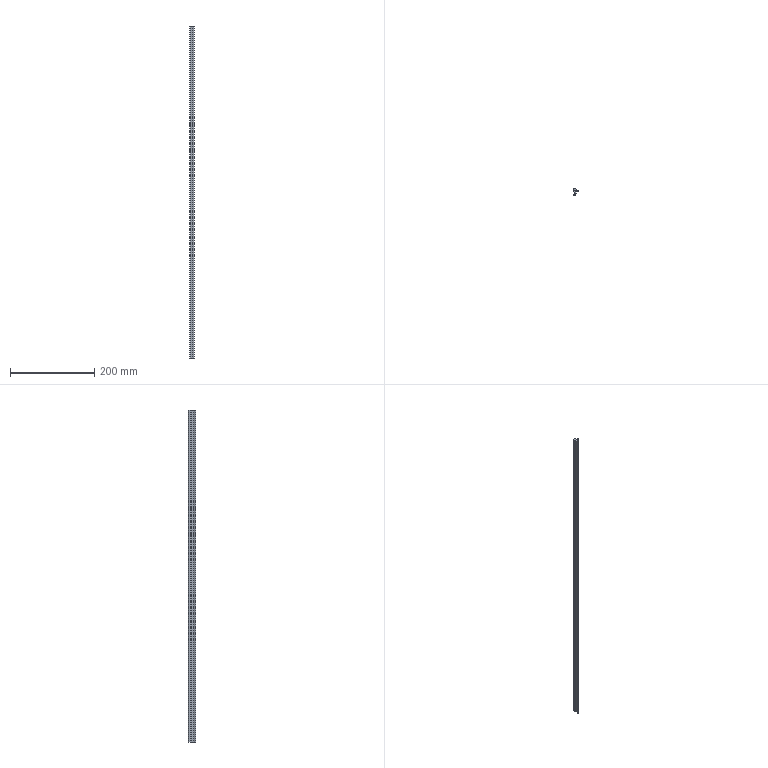Part | SolidWorks | features BaseBody 1, MoveFace 1 | 1 solid | 20 faces | box 10.8 x 17.5 x 788 mm | volume 62095 mm3 | cylinder 11 | plane 9 | commonest cylinder face diameters 1.6 x2 14 x2 0.4 x1 0.6 x1 0.8 x1 2.6 x1
STEP:
#1=CARTESIAN_POINT('',(-3.236,-11.055,688.));
#2=VERTEX_POINT('',#1);
#3=CARTESIAN_POINT('',(-4.3,-10.3,688.));
#4=VERTEX_POINT('',#3);
#5=CARTESIAN_POINT('',(-3.5,-10.3,688.));
#6=DIRECTION('',(0.,0.,-1.));
#7=DIRECTION('',(1.,0.,0.));
#8=AXIS2_PLACEMENT_3D('',#5,#6,#7);
#9=CIRCLE('',#8,0.8);
#10=EDGE_CURVE('',#2,#4,#9,.T.);
#11=ORIENTED_EDGE('',*,*,#10,.T.);
#12=CARTESIAN_POINT('',(-4.3,-10.3,-100.));
#13=VERTEX_POINT('',#12);
#14=CARTESIAN_POINT('',(-4.3,-10.3,-100.));
#15=DIRECTION('',(0.,0.,-1.));
#16=VECTOR('',#15,1000.);
#17=LINE('',#14,#16);
#18=EDGE_CURVE('',#4,#13,#17,.T.);
#19=ORIENTED_EDGE('',*,*,#18,.T.);
#20=CARTESIAN_POINT('',(-3.236,-11.055,-100.));
#21=VERTEX_POINT('',#20);
#22=CARTESIAN_POINT('',(-3.5,-10.3,-100.));
#23=DIRECTION('',(0.,0.,1.));
#24=DIRECTION('',(-1.,0.,0.));
#25=AXIS2_PLACEMENT_3D('',#22,#23,#24);
#26=CIRCLE('',#25,0.8);
#27=EDGE_CURVE('',#13,#21,#26,.T.);
#28=ORIENTED_EDGE('',*,*,#27,.T.);
#29=CARTESIAN_POINT('',(-3.236,-11.055,-100.));
#30=DIRECTION('',(0.,0.,-1.));
#31=VECTOR('',#30,1000.);
#32=LINE('',#29,#31);
#33=EDGE_CURVE('',#2,#21,#32,.T.);
#34=ORIENTED_EDGE('',*,*,#33,.F.);
#35=EDGE_LOOP('',(#11,#19,#28,#34));
#36=FACE_OUTER_BOUND('',#35,.T.);
#37=CARTESIAN_POINT('',(-3.5,-10.3,-100.));
#38=DIRECTION('',(0.,0.,-1.));
#39=DIRECTION('',(-1.,0.,0.));
#40=AXIS2_PLACEMENT_3D('',#37,#38,#39);
#41=CYLINDRICAL_SURFACE('',#40,0.8);
#42=ADVANCED_FACE('',(#36),#41,.T.);
#43=CARTESIAN_POINT('',(1.184,-6.397,-100.));
#44=VERTEX_POINT('',#43);
#45=CARTESIAN_POINT('',(-5.702,-4.29,-100.));
#46=DIRECTION('',(0.,0.,1.));
#47=DIRECTION('',(-1.,0.,0.));
#48=AXIS2_PLACEMENT_3D('',#45,#46,#47);
#49=CIRCLE('',#48,7.201);
#50=EDGE_CURVE('',#21,#44,#49,.T.);
#51=ORIENTED_EDGE('',*,*,#50,.T.);
#52=CARTESIAN_POINT('',(1.184,-6.397,688.));
#53=VERTEX_POINT('',#52);
#54=CARTESIAN_POINT('',(1.184,-6.397,-100.));
#55=DIRECTION('',(0.,0.,1.));
#56=VECTOR('',#55,1000.);
#57=LINE('',#54,#56);
#58=EDGE_CURVE('',#44,#53,#57,.T.);
#59=ORIENTED_EDGE('',*,*,#58,.T.);
#60=CARTESIAN_POINT('',(-5.702,-4.29,688.));
#61=DIRECTION('',(0.,0.,-1.));
#62=DIRECTION('',(1.,0.,0.));
#63=AXIS2_PLACEMENT_3D('',#60,#61,#62);
#64=CIRCLE('',#63,7.201);
#65=EDGE_CURVE('',#53,#2,#64,.T.);
#66=ORIENTED_EDGE('',*,*,#65,.T.);
#67=ORIENTED_EDGE('',*,*,#33,.T.);
#68=EDGE_LOOP('',(#51,#59,#66,#67));
#69=FACE_OUTER_BOUND('',#68,.T.);
#70=CARTESIAN_POINT('',(-5.702,-4.29,-100.));
#71=DIRECTION('',(0.,0.,-1.));
#72=DIRECTION('',(-1.,0.,0.));
#73=AXIS2_PLACEMENT_3D('',#70,#71,#72);
#74=CYLINDRICAL_SURFACE('',#73,7.201);
#75=ADVANCED_FACE('',(#69),#74,.T.);
#76=CARTESIAN_POINT('',(0.9,-6.,-100.));
#77=VERTEX_POINT('',#76);
#78=CARTESIAN_POINT('',(0.9,-6.3,-100.));
#79=DIRECTION('',(0.,0.,1.));
#80=DIRECTION('',(-1.,0.,0.));
#81=AXIS2_PLACEMENT_3D('',#78,#79,#80);
#82=CIRCLE('',#81,0.3);
#83=EDGE_CURVE('',#44,#77,#82,.T.);
#84=ORIENTED_EDGE('',*,*,#83,.T.);
#85=CARTESIAN_POINT('',(0.9,-6.,688.));
#86=VERTEX_POINT('',#85);
#87=CARTESIAN_POINT('',(0.9,-6.,-100.));
#88=DIRECTION('',(0.,0.,1.));
#89=VECTOR('',#88,1000.);
#90=LINE('',#87,#89);
#91=EDGE_CURVE('',#77,#86,#90,.T.);
#92=ORIENTED_EDGE('',*,*,#91,.T.);
#93=CARTESIAN_POINT('',(0.9,-6.3,688.));
#94=DIRECTION('',(0.,0.,-1.));
#95=DIRECTION('',(1.,0.,0.));
#96=AXIS2_PLACEMENT_3D('',#93,#94,#95);
#97=CIRCLE('',#96,0.3);
#98=EDGE_CURVE('',#86,#53,#97,.T.);
#99=ORIENTED_EDGE('',*,*,#98,.T.);
#100=ORIENTED_EDGE('',*,*,#58,.F.);
#101=EDGE_LOOP('',(#84,#92,#99,#100));
#102=FACE_OUTER_BOUND('',#101,.T.);
#103=CARTESIAN_POINT('',(0.9,-6.3,-100.));
#104=DIRECTION('',(0.,0.,-1.));
#105=DIRECTION('',(-1.,0.,0.));
#106=AXIS2_PLACEMENT_3D('',#103,#104,#105);
#107=CYLINDRICAL_SURFACE('',#106,0.3);
#108=ADVANCED_FACE('',(#102),#107,.T.);
#109=CARTESIAN_POINT('',(-2.5,-0.5,-100.));
#110=VERTEX_POINT('',#109);
#111=CARTESIAN_POINT('',(-2.5,-6.153,-100.));
#112=VERTEX_POINT('',#111);
#113=CARTESIAN_POINT('',(-2.5,-6.397,-100.));
#114=DIRECTION('',(0.,-1.,0.));
#115=VECTOR('',#114,1000.);
#116=LINE('',#113,#115);
#117=EDGE_CURVE('',#110,#112,#116,.T.);
#118=ORIENTED_EDGE('',*,*,#117,.F.);
#119=CARTESIAN_POINT('',(-4.2,1.695,-100.));
#120=VERTEX_POINT('',#119);
#121=CARTESIAN_POINT('',(-1.701,1.875,-100.));
#122=DIRECTION('',(0.,0.,1.));
#123=DIRECTION('',(-1.,0.,0.));
#124=AXIS2_PLACEMENT_3D('',#121,#122,#123);
#125=CIRCLE('',#124,2.506);
#126=EDGE_CURVE('',#120,#110,#125,.T.);
#127=ORIENTED_EDGE('',*,*,#126,.F.);
#128=CARTESIAN_POINT('',(-4.2,5.1,-100.));
#129=VERTEX_POINT('',#128);
#130=CARTESIAN_POINT('',(-4.2,-6.397,-100.));
#131=DIRECTION('',(0.,-1.,0.));
#132=VECTOR('',#131,1000.);
#133=LINE('',#130,#132);
#134=EDGE_CURVE('',#129,#120,#133,.T.);
#135=ORIENTED_EDGE('',*,*,#134,.F.);
#136=CARTESIAN_POINT('',(-2.892,6.4,-100.));
#137=VERTEX_POINT('',#136);
#138=CARTESIAN_POINT('',(-2.9,5.1,-100.));
#139=DIRECTION('',(0.,0.,1.));
#140=DIRECTION('',(-1.,0.,0.));
#141=AXIS2_PLACEMENT_3D('',#138,#139,#140);
#142=CIRCLE('',#141,1.3);
#143=EDGE_CURVE('',#137,#129,#142,.T.);
#144=ORIENTED_EDGE('',*,*,#143,.F.);
#145=CARTESIAN_POINT('',(0.5,5.5,-100.));
#146=VERTEX_POINT('',#145);
#147=CARTESIAN_POINT('',(-2.934,-0.5999,-100.));
#148=DIRECTION('',(0.,0.,1.));
#149=DIRECTION('',(-1.,0.,0.));
#150=AXIS2_PLACEMENT_3D('',#147,#148,#149);
#151=CIRCLE('',#150,7.);
#152=EDGE_CURVE('',#146,#137,#151,.T.);
#153=ORIENTED_EDGE('',*,*,#152,.F.);
#154=CARTESIAN_POINT('',(5.5,1.7,-100.));
#155=VERTEX_POINT('',#154);
#156=CARTESIAN_POINT('',(5.5,1.7,-100.));
#157=DIRECTION('',(-0.7962,0.6051,0.));
#158=VECTOR('',#157,1000.);
#159=LINE('',#156,#158);
#160=EDGE_CURVE('',#155,#146,#159,.T.);
#161=ORIENTED_EDGE('',*,*,#160,.F.);
#162=CARTESIAN_POINT('',(6.458,-0.2215,-100.));
#163=VERTEX_POINT('',#162);
#164=CARTESIAN_POINT('',(6.458,-0.2215,-100.));
#165=DIRECTION('',(-0.4462,0.8949,0.));
#166=VECTOR('',#165,1000.);
#167=LINE('',#164,#166);
#168=EDGE_CURVE('',#163,#155,#167,.T.);
#169=ORIENTED_EDGE('',*,*,#168,.F.);
#170=CARTESIAN_POINT('',(5.895,-0.7433,-100.));
#171=VERTEX_POINT('',#170);
#172=CARTESIAN_POINT('',(6.1,-0.4,-100.));
#173=DIRECTION('',(0.,0.,1.));
#174=DIRECTION('',(-1.,0.,0.));
#175=AXIS2_PLACEMENT_3D('',#172,#173,#174);
#176=CIRCLE('',#175,0.4);
#177=EDGE_CURVE('',#171,#163,#176,.T.);
#178=ORIENTED_EDGE('',*,*,#177,.F.);
#179=CARTESIAN_POINT('',(3.,0.,-100.));
#180=VERTEX_POINT('',#179);
#181=CARTESIAN_POINT('',(2.746,-6.995,-100.));
#182=DIRECTION('',(0.,0.,-1.));
#183=DIRECTION('',(-1.,0.,0.));
#184=AXIS2_PLACEMENT_3D('',#181,#182,#183);
#185=CIRCLE('',#184,7.);
#186=EDGE_CURVE('',#180,#171,#185,.T.);
#187=ORIENTED_EDGE('',*,*,#186,.F.);
#188=CARTESIAN_POINT('',(0.,0.,-100.));
#189=VERTEX_POINT('',#188);
#190=CARTESIAN_POINT('',(-6.814,0.,-100.));
#191=DIRECTION('',(1.,0.,0.));
#192=VECTOR('',#191,1000.);
#193=LINE('',#190,#192);
#194=EDGE_CURVE('',#189,#180,#193,.T.);
#195=ORIENTED_EDGE('',*,*,#194,.F.);
#196=CARTESIAN_POINT('',(0.,-5.8,-100.));
#197=VERTEX_POINT('',#196);
#198=CARTESIAN_POINT('',(0.,-6.397,-100.));
#199=DIRECTION('',(0.,1.,0.));
#200=VECTOR('',#199,1000.);
#201=LINE('',#198,#200);
#202=EDGE_CURVE('',#197,#189,#201,.T.);
#203=ORIENTED_EDGE('',*,*,#202,.F.);
#204=CARTESIAN_POINT('',(0.2,-6.,-100.));
#205=VERTEX_POINT('',#204);
#206=CARTESIAN_POINT('',(0.2,-5.8,-100.));
#207=DIRECTION('',(0.,0.,1.));
#208=DIRECTION('',(-1.,0.,0.));
#209=AXIS2_PLACEMENT_3D('',#206,#207,#208);
#210=CIRCLE('',#209,0.2);
#211=EDGE_CURVE('',#197,#205,#210,.T.);
#212=ORIENTED_EDGE('',*,*,#211,.T.);
#213=CARTESIAN_POINT('',(-6.814,-6.,-100.));
#214=DIRECTION('',(-1.,0.,0.));
#215=VECTOR('',#214,1000.);
#216=LINE('',#213,#215);
#217=EDGE_CURVE('',#77,#205,#216,.T.);
#218=ORIENTED_EDGE('',*,*,#217,.F.);
#219=ORIENTED_EDGE('',*,*,#83,.F.);
#220=ORIENTED_EDGE('',*,*,#50,.F.);
#221=ORIENTED_EDGE('',*,*,#27,.F.);
#222=CARTESIAN_POINT('',(-3.998,-9.674,-100.));
#223=VERTEX_POINT('',#222);
#224=CARTESIAN_POINT('',(-3.5,-10.3,-100.));
#225=DIRECTION('',(0.,0.,1.));
#226=DIRECTION('',(-1.,0.,0.));
#227=AXIS2_PLACEMENT_3D('',#224,#225,#226);
#228=CIRCLE('',#227,0.8);
#229=EDGE_CURVE('',#223,#13,#228,.T.);
#230=ORIENTED_EDGE('',*,*,#229,.F.);
#231=CARTESIAN_POINT('',(-6.814,-6.397,-100.));
#232=DIRECTION('',(0.,0.,-1.));
#233=DIRECTION('',(-1.,0.,0.));
#234=AXIS2_PLACEMENT_3D('',#231,#232,#233);
#235=CIRCLE('',#234,4.321);
#236=EDGE_CURVE('',#112,#223,#235,.T.);
#237=ORIENTED_EDGE('',*,*,#236,.F.);
#238=EDGE_LOOP('',(#118,#127,#135,#144,#153,#161,#169,#178,#187,#195,#203,#212,#218,#219,#220,#221,#230,#237));
#239=FACE_OUTER_BOUND('',#238,.T.);
#240=CARTESIAN_POINT('',(-6.814,-6.397,-100.));
#241=DIRECTION('',(0.,0.,1.));
#242=DIRECTION('',(1.,0.,0.));
#243=AXIS2_PLACEMENT_3D('',#240,#241,#242);
#244=PLANE('',#243);
#245=ADVANCED_FACE('',(#239),#244,.F.);
#246=ORIENTED_EDGE('',*,*,#18,.F.);
#247=CARTESIAN_POINT('',(-3.998,-9.674,688.));
#248=VERTEX_POINT('',#247);
#249=CARTESIAN_POINT('',(-3.5,-10.3,688.));
#250=DIRECTION('',(0.,0.,-1.));
#251=DIRECTION('',(1.,0.,0.));
#252=AXIS2_PLACEMENT_3D('',#249,#250,#251);
#253=CIRCLE('',#252,0.8);
#254=EDGE_CURVE('',#4,#248,#253,.T.);
#255=ORIENTED_EDGE('',*,*,#254,.T.);
#256=CARTESIAN_POINT('',(-3.998,-9.674,-100.));
#257=DIRECTION('',(0.,0.,-1.));
#258=VECTOR('',#257,1000.);
#259=LINE('',#256,#258);
#260=EDGE_CURVE('',#248,#223,#259,.T.);
#261=ORIENTED_EDGE('',*,*,#260,.T.);
#262=ORIENTED_EDGE('',*,*,#229,.T.);
#263=EDGE_LOOP('',(#246,#255,#261,#262));
#264=FACE_OUTER_BOUND('',#263,.T.);
#265=CARTESIAN_POINT('',(-3.5,-10.3,-100.));
#266=DIRECTION('',(0.,0.,-1.));
#267=DIRECTION('',(-1.,0.,0.));
#268=AXIS2_PLACEMENT_3D('',#265,#266,#267);
#269=CYLINDRICAL_SURFACE('',#268,0.8);
#270=ADVANCED_FACE('',(#264),#269,.T.);
#271=CARTESIAN_POINT('',(-4.2,1.695,688.));
#272=VERTEX_POINT('',#271);
#273=CARTESIAN_POINT('',(-2.5,-0.5,688.));
#274=VERTEX_POINT('',#273);
#275=CARTESIAN_POINT('',(-1.701,1.875,688.));
#276=DIRECTION('',(0.,0.,1.));
#277=DIRECTION('',(1.,0.,0.));
#278=AXIS2_PLACEMENT_3D('',#275,#276,#277);
#279=CIRCLE('',#278,2.506);
#280=EDGE_CURVE('',#272,#274,#279,.T.);
#281=ORIENTED_EDGE('',*,*,#280,.T.);
#282=CARTESIAN_POINT('',(-2.5,-6.153,688.));
#283=VERTEX_POINT('',#282);
#284=CARTESIAN_POINT('',(-2.5,-6.397,688.));
#285=DIRECTION('',(0.,-1.,0.));
#286=VECTOR('',#285,1000.);
#287=LINE('',#284,#286);
#288=EDGE_CURVE('',#274,#283,#287,.T.);
#289=ORIENTED_EDGE('',*,*,#288,.T.);
#290=CARTESIAN_POINT('',(-6.814,-6.397,688.));
#291=DIRECTION('',(0.,0.,-1.));
#292=DIRECTION('',(1.,0.,0.));
#293=AXIS2_PLACEMENT_3D('',#290,#291,#292);
#294=CIRCLE('',#293,4.321);
#295=EDGE_CURVE('',#283,#248,#294,.T.);
#296=ORIENTED_EDGE('',*,*,#295,.T.);
#297=ORIENTED_EDGE('',*,*,#254,.F.);
#298=ORIENTED_EDGE('',*,*,#10,.F.);
#299=ORIENTED_EDGE('',*,*,#65,.F.);
#300=ORIENTED_EDGE('',*,*,#98,.F.);
#301=CARTESIAN_POINT('',(0.2,-6.,688.));
#302=VERTEX_POINT('',#301);
#303=CARTESIAN_POINT('',(-6.814,-6.,688.));
#304=DIRECTION('',(-1.,0.,0.));
#305=VECTOR('',#304,1000.);
#306=LINE('',#303,#305);
#307=EDGE_CURVE('',#86,#302,#306,.T.);
#308=ORIENTED_EDGE('',*,*,#307,.T.);
#309=CARTESIAN_POINT('',(0.,-5.8,688.));
#310=VERTEX_POINT('',#309);
#311=CARTESIAN_POINT('',(0.2,-5.8,688.));
#312=DIRECTION('',(0.,0.,-1.));
#313=DIRECTION('',(1.,0.,0.));
#314=AXIS2_PLACEMENT_3D('',#311,#312,#313);
#315=CIRCLE('',#314,0.2);
#316=EDGE_CURVE('',#302,#310,#315,.T.);
#317=ORIENTED_EDGE('',*,*,#316,.T.);
#318=CARTESIAN_POINT('',(0.,0.,688.));
#319=VERTEX_POINT('',#318);
#320=CARTESIAN_POINT('',(0.,-6.397,688.));
#321=DIRECTION('',(0.,1.,0.));
#322=VECTOR('',#321,1000.);
#323=LINE('',#320,#322);
#324=EDGE_CURVE('',#310,#319,#323,.T.);
#325=ORIENTED_EDGE('',*,*,#324,.T.);
#326=CARTESIAN_POINT('',(3.,0.,688.));
#327=VERTEX_POINT('',#326);
#328=CARTESIAN_POINT('',(-6.814,0.,688.));
#329=DIRECTION('',(1.,0.,0.));
#330=VECTOR('',#329,1000.);
#331=LINE('',#328,#330);
#332=EDGE_CURVE('',#319,#327,#331,.T.);
#333=ORIENTED_EDGE('',*,*,#332,.T.);
#334=CARTESIAN_POINT('',(5.895,-0.7433,688.));
#335=VERTEX_POINT('',#334);
#336=CARTESIAN_POINT('',(2.746,-6.995,688.));
#337=DIRECTION('',(0.,0.,-1.));
#338=DIRECTION('',(1.,0.,0.));
#339=AXIS2_PLACEMENT_3D('',#336,#337,#338);
#340=CIRCLE('',#339,7.);
#341=EDGE_CURVE('',#327,#335,#340,.T.);
#342=ORIENTED_EDGE('',*,*,#341,.T.);
#343=CARTESIAN_POINT('',(6.458,-0.2215,688.));
#344=VERTEX_POINT('',#343);
#345=CARTESIAN_POINT('',(6.1,-0.4,688.));
#346=DIRECTION('',(0.,0.,-1.));
#347=DIRECTION('',(1.,0.,0.));
#348=AXIS2_PLACEMENT_3D('',#345,#346,#347);
#349=CIRCLE('',#348,0.4);
#350=EDGE_CURVE('',#344,#335,#349,.T.);
#351=ORIENTED_EDGE('',*,*,#350,.F.);
#352=CARTESIAN_POINT('',(5.5,1.7,688.));
#353=VERTEX_POINT('',#352);
#354=CARTESIAN_POINT('',(6.282,0.1323,688.));
#355=DIRECTION('',(-0.4462,0.8949,0.));
#356=VECTOR('',#355,1000.);
#357=LINE('',#354,#356);
#358=EDGE_CURVE('',#344,#353,#357,.T.);
#359=ORIENTED_EDGE('',*,*,#358,.T.);
#360=CARTESIAN_POINT('',(0.5,5.5,688.));
#361=VERTEX_POINT('',#360);
#362=CARTESIAN_POINT('',(1.595,4.668,688.));
#363=DIRECTION('',(-0.7962,0.6051,0.));
#364=VECTOR('',#363,1000.);
#365=LINE('',#362,#364);
#366=EDGE_CURVE('',#353,#361,#365,.T.);
#367=ORIENTED_EDGE('',*,*,#366,.T.);
#368=CARTESIAN_POINT('',(-2.892,6.4,688.));
#369=VERTEX_POINT('',#368);
#370=CARTESIAN_POINT('',(-2.934,-0.5999,688.));
#371=DIRECTION('',(0.,0.,1.));
#372=DIRECTION('',(1.,0.,0.));
#373=AXIS2_PLACEMENT_3D('',#370,#371,#372);
#374=CIRCLE('',#373,7.);
#375=EDGE_CURVE('',#361,#369,#374,.T.);
#376=ORIENTED_EDGE('',*,*,#375,.T.);
#377=CARTESIAN_POINT('',(-4.2,5.1,688.));
#378=VERTEX_POINT('',#377);
#379=CARTESIAN_POINT('',(-2.9,5.1,688.));
#380=DIRECTION('',(0.,0.,1.));
#381=DIRECTION('',(1.,0.,0.));
#382=AXIS2_PLACEMENT_3D('',#379,#380,#381);
#383=CIRCLE('',#382,1.3);
#384=EDGE_CURVE('',#369,#378,#383,.T.);
#385=ORIENTED_EDGE('',*,*,#384,.T.);
#386=CARTESIAN_POINT('',(-4.2,-6.397,688.));
#387=DIRECTION('',(0.,-1.,0.));
#388=VECTOR('',#387,1000.);
#389=LINE('',#386,#388);
#390=EDGE_CURVE('',#378,#272,#389,.T.);
#391=ORIENTED_EDGE('',*,*,#390,.T.);
#392=EDGE_LOOP('',(#281,#289,#296,#297,#298,#299,#300,#308,#317,#325,#333,#342,#351,#359,#367,#376,#385,#391));
#393=FACE_OUTER_BOUND('',#392,.T.);
#394=CARTESIAN_POINT('',(-6.814,-6.397,688.));
#395=DIRECTION('',(0.,0.,1.));
#396=DIRECTION('',(1.,0.,0.));
#397=AXIS2_PLACEMENT_3D('',#394,#395,#396);
#398=PLANE('',#397);
#399=ADVANCED_FACE('',(#393),#398,.T.);
#400=ORIENTED_EDGE('',*,*,#217,.T.);
#401=CARTESIAN_POINT('',(0.2,-6.,-100.));
#402=DIRECTION('',(0.,0.,1.));
#403=VECTOR('',#402,1000.);
#404=LINE('',#401,#403);
#405=EDGE_CURVE('',#205,#302,#404,.T.);
#406=ORIENTED_EDGE('',*,*,#405,.T.);
#407=ORIENTED_EDGE('',*,*,#307,.F.);
#408=ORIENTED_EDGE('',*,*,#91,.F.);
#409=EDGE_LOOP('',(#400,#406,#407,#408));
#410=FACE_OUTER_BOUND('',#409,.T.);
#411=CARTESIAN_POINT('',(0.9,-6.,-100.));
#412=DIRECTION('',(0.,1.,0.));
#413=DIRECTION('',(0.,0.,1.));
#414=AXIS2_PLACEMENT_3D('',#411,#412,#413);
#415=PLANE('',#414);
#416=ADVANCED_FACE('',(#410),#415,.T.);
#417=CARTESIAN_POINT('',(-2.5,-6.153,-100.));
#418=DIRECTION('',(0.,0.,1.));
#419=VECTOR('',#418,1000.);
#420=LINE('',#417,#419);
#421=EDGE_CURVE('',#112,#283,#420,.T.);
#422=ORIENTED_EDGE('',*,*,#421,.F.);
#423=ORIENTED_EDGE('',*,*,#236,.T.);
#424=ORIENTED_EDGE('',*,*,#260,.F.);
#425=ORIENTED_EDGE('',*,*,#295,.F.);
#426=EDGE_LOOP('',(#422,#423,#424,#425));
#427=FACE_OUTER_BOUND('',#426,.T.);
#428=CARTESIAN_POINT('',(-6.814,-6.397,-100.));
#429=DIRECTION('',(0.,0.,-1.));
#430=DIRECTION('',(-1.,0.,0.));
#431=AXIS2_PLACEMENT_3D('',#428,#429,#430);
#432=CYLINDRICAL_SURFACE('',#431,4.321);
#433=ADVANCED_FACE('',(#427),#432,.F.);
#434=ORIENTED_EDGE('',*,*,#117,.T.);
#435=ORIENTED_EDGE('',*,*,#421,.T.);
#436=ORIENTED_EDGE('',*,*,#288,.F.);
#437=CARTESIAN_POINT('',(-2.5,-0.5,-100.));
#438=DIRECTION('',(0.,0.,-1.));
#439=VECTOR('',#438,1000.);
#440=LINE('',#437,#439);
#441=EDGE_CURVE('',#274,#110,#440,.T.);
#442=ORIENTED_EDGE('',*,*,#441,.T.);
#443=EDGE_LOOP('',(#434,#435,#436,#442));
#444=FACE_OUTER_BOUND('',#443,.T.);
#445=CARTESIAN_POINT('',(-2.5,-0.5,-100.));
#446=DIRECTION('',(-1.,0.,0.));
#447=DIRECTION('',(0.,0.,1.));
#448=AXIS2_PLACEMENT_3D('',#445,#446,#447);
#449=PLANE('',#448);
#450=ADVANCED_FACE('',(#444),#449,.T.);
#451=ORIENTED_EDGE('',*,*,#126,.T.);
#452=ORIENTED_EDGE('',*,*,#441,.F.);
#453=ORIENTED_EDGE('',*,*,#280,.F.);
#454=CARTESIAN_POINT('',(-4.2,1.695,-100.));
#455=DIRECTION('',(0.,0.,-1.));
#456=VECTOR('',#455,1000.);
#457=LINE('',#454,#456);
#458=EDGE_CURVE('',#272,#120,#457,.T.);
#459=ORIENTED_EDGE('',*,*,#458,.T.);
#460=EDGE_LOOP('',(#451,#452,#453,#459));
#461=FACE_OUTER_BOUND('',#460,.T.);
#462=CARTESIAN_POINT('',(-1.701,1.875,-100.));
#463=DIRECTION('',(0.,0.,-1.));
#464=DIRECTION('',(-1.,0.,0.));
#465=AXIS2_PLACEMENT_3D('',#462,#463,#464);
#466=CYLINDRICAL_SURFACE('',#465,2.506);
#467=ADVANCED_FACE('',(#461),#466,.T.);
#468=ORIENTED_EDGE('',*,*,#134,.T.);
#469=ORIENTED_EDGE('',*,*,#458,.F.);
#470=ORIENTED_EDGE('',*,*,#390,.F.);
#471=CARTESIAN_POINT('',(-4.2,5.1,-100.));
#472=DIRECTION('',(0.,0.,-1.));
#473=VECTOR('',#472,1000.);
#474=LINE('',#471,#473);
#475=EDGE_CURVE('',#378,#129,#474,.T.);
#476=ORIENTED_EDGE('',*,*,#475,.T.);
#477=EDGE_LOOP('',(#468,#469,#470,#476));
#478=FACE_OUTER_BOUND('',#477,.T.);
#479=CARTESIAN_POINT('',(-4.2,5.1,-100.));
#480=DIRECTION('',(-1.,0.,0.));
#481=DIRECTION('',(0.,0.,1.));
#482=AXIS2_PLACEMENT_3D('',#479,#480,#481);
#483=PLANE('',#482);
#484=ADVANCED_FACE('',(#478),#483,.T.);
#485=ORIENTED_EDGE('',*,*,#143,.T.);
#486=ORIENTED_EDGE('',*,*,#475,.F.);
#487=ORIENTED_EDGE('',*,*,#384,.F.);
#488=CARTESIAN_POINT('',(-2.892,6.4,-100.));
#489=DIRECTION('',(0.,0.,-1.));
#490=VECTOR('',#489,1000.);
#491=LINE('',#488,#490);
#492=EDGE_CURVE('',#369,#137,#491,.T.);
#493=ORIENTED_EDGE('',*,*,#492,.T.);
#494=EDGE_LOOP('',(#485,#486,#487,#493));
#495=FACE_OUTER_BOUND('',#494,.T.);
#496=CARTESIAN_POINT('',(-2.9,5.1,-100.));
#497=DIRECTION('',(0.,0.,-1.));
#498=DIRECTION('',(-1.,0.,0.));
#499=AXIS2_PLACEMENT_3D('',#496,#497,#498);
#500=CYLINDRICAL_SURFACE('',#499,1.3);
#501=ADVANCED_FACE('',(#495),#500,.T.);
#502=ORIENTED_EDGE('',*,*,#152,.T.);
#503=ORIENTED_EDGE('',*,*,#492,.F.);
#504=ORIENTED_EDGE('',*,*,#375,.F.);
#505=CARTESIAN_POINT('',(0.5,5.5,-100.));
#506=DIRECTION('',(0.,0.,-1.));
#507=VECTOR('',#506,1000.);
#508=LINE('',#505,#507);
#509=EDGE_CURVE('',#361,#146,#508,.T.);
#510=ORIENTED_EDGE('',*,*,#509,.T.);
#511=EDGE_LOOP('',(#502,#503,#504,#510));
#512=FACE_OUTER_BOUND('',#511,.T.);
#513=CARTESIAN_POINT('',(-2.934,-0.5999,-100.));
#514=DIRECTION('',(0.,0.,-1.));
#515=DIRECTION('',(-1.,0.,0.));
#516=AXIS2_PLACEMENT_3D('',#513,#514,#515);
#517=CYLINDRICAL_SURFACE('',#516,7.);
#518=ADVANCED_FACE('',(#512),#517,.T.);
#519=ORIENTED_EDGE('',*,*,#160,.T.);
#520=ORIENTED_EDGE('',*,*,#509,.F.);
#521=ORIENTED_EDGE('',*,*,#366,.F.);
#522=CARTESIAN_POINT('',(5.5,1.7,-100.));
#523=DIRECTION('',(0.,0.,-1.));
#524=VECTOR('',#523,1000.);
#525=LINE('',#522,#524);
#526=EDGE_CURVE('',#353,#155,#525,.T.);
#527=ORIENTED_EDGE('',*,*,#526,.T.);
#528=EDGE_LOOP('',(#519,#520,#521,#527));
#529=FACE_OUTER_BOUND('',#528,.T.);
#530=CARTESIAN_POINT('',(5.5,1.7,-100.));
#531=DIRECTION('',(0.6051,0.7962,0.));
#532=DIRECTION('',(-0.7962,0.6051,0.));
#533=AXIS2_PLACEMENT_3D('',#530,#531,#532);
#534=PLANE('',#533);
#535=ADVANCED_FACE('',(#529),#534,.T.);
#536=ORIENTED_EDGE('',*,*,#168,.T.);
#537=ORIENTED_EDGE('',*,*,#526,.F.);
#538=ORIENTED_EDGE('',*,*,#358,.F.);
#539=CARTESIAN_POINT('',(6.458,-0.2215,-100.));
#540=DIRECTION('',(0.,0.,-1.));
#541=VECTOR('',#540,1000.);
#542=LINE('',#539,#541);
#543=EDGE_CURVE('',#344,#163,#542,.T.);
#544=ORIENTED_EDGE('',*,*,#543,.T.);
#545=EDGE_LOOP('',(#536,#537,#538,#544));
#546=FACE_OUTER_BOUND('',#545,.T.);
#547=CARTESIAN_POINT('',(6.458,-0.2215,-100.));
#548=DIRECTION('',(0.8949,0.4462,0.));
#549=DIRECTION('',(-0.4462,0.8949,0.));
#550=AXIS2_PLACEMENT_3D('',#547,#548,#549);
#551=PLANE('',#550);
#552=ADVANCED_FACE('',(#546),#551,.T.);
#553=CARTESIAN_POINT('',(3.,0.,-100.));
#554=DIRECTION('',(0.,0.,1.));
#555=VECTOR('',#554,1000.);
#556=LINE('',#553,#555);
#557=EDGE_CURVE('',#180,#327,#556,.T.);
#558=ORIENTED_EDGE('',*,*,#557,.F.);
#559=ORIENTED_EDGE('',*,*,#186,.T.);
#560=CARTESIAN_POINT('',(5.895,-0.7433,-100.));
#561=DIRECTION('',(0.,0.,-1.));
#562=VECTOR('',#561,1000.);
#563=LINE('',#560,#562);
#564=EDGE_CURVE('',#335,#171,#563,.T.);
#565=ORIENTED_EDGE('',*,*,#564,.F.);
#566=ORIENTED_EDGE('',*,*,#341,.F.);
#567=EDGE_LOOP('',(#558,#559,#565,#566));
#568=FACE_OUTER_BOUND('',#567,.T.);
#569=CARTESIAN_POINT('',(2.746,-6.995,-100.));
#570=DIRECTION('',(0.,0.,-1.));
#571=DIRECTION('',(-1.,0.,0.));
#572=AXIS2_PLACEMENT_3D('',#569,#570,#571);
#573=CYLINDRICAL_SURFACE('',#572,7.);
#574=ADVANCED_FACE('',(#568),#573,.F.);
#575=ORIENTED_EDGE('',*,*,#194,.T.);
#576=ORIENTED_EDGE('',*,*,#557,.T.);
#577=ORIENTED_EDGE('',*,*,#332,.F.);
#578=CARTESIAN_POINT('',(0.,0.,-100.));
#579=DIRECTION('',(0.,0.,-1.));
#580=VECTOR('',#579,1000.);
#581=LINE('',#578,#580);
#582=EDGE_CURVE('',#319,#189,#581,.T.);
#583=ORIENTED_EDGE('',*,*,#582,.T.);
#584=EDGE_LOOP('',(#575,#576,#577,#583));
#585=FACE_OUTER_BOUND('',#584,.T.);
#586=CARTESIAN_POINT('',(0.,0.,-100.));
#587=DIRECTION('',(0.,-1.,0.));
#588=DIRECTION('',(0.,0.,-1.));
#589=AXIS2_PLACEMENT_3D('',#586,#587,#588);
#590=PLANE('',#589);
#591=ADVANCED_FACE('',(#585),#590,.T.);
#592=ORIENTED_EDGE('',*,*,#202,.T.);
#593=ORIENTED_EDGE('',*,*,#582,.F.);
#594=ORIENTED_EDGE('',*,*,#324,.F.);
#595=CARTESIAN_POINT('',(0.,-5.8,-100.));
#596=DIRECTION('',(0.,0.,-1.));
#597=VECTOR('',#596,1000.);
#598=LINE('',#595,#597);
#599=EDGE_CURVE('',#310,#197,#598,.T.);
#600=ORIENTED_EDGE('',*,*,#599,.T.);
#601=EDGE_LOOP('',(#592,#593,#594,#600));
#602=FACE_OUTER_BOUND('',#601,.T.);
#603=CARTESIAN_POINT('',(0.,-5.8,-100.));
#604=DIRECTION('',(1.,0.,0.));
#605=DIRECTION('',(0.,0.,-1.));
#606=AXIS2_PLACEMENT_3D('',#603,#604,#605);
#607=PLANE('',#606);
#608=ADVANCED_FACE('',(#602),#607,.T.);
#609=ORIENTED_EDGE('',*,*,#405,.F.);
#610=ORIENTED_EDGE('',*,*,#211,.F.);
#611=ORIENTED_EDGE('',*,*,#599,.F.);
#612=ORIENTED_EDGE('',*,*,#316,.F.);
#613=EDGE_LOOP('',(#609,#610,#611,#612));
#614=FACE_OUTER_BOUND('',#613,.T.);
#615=CARTESIAN_POINT('',(0.2,-5.8,-100.));
#616=DIRECTION('',(0.,0.,-1.));
#617=DIRECTION('',(-1.,0.,0.));
#618=AXIS2_PLACEMENT_3D('',#615,#616,#617);
#619=CYLINDRICAL_SURFACE('',#618,0.2);
#620=ADVANCED_FACE('',(#614),#619,.F.);
#621=ORIENTED_EDGE('',*,*,#177,.T.);
#622=ORIENTED_EDGE('',*,*,#543,.F.);
#623=ORIENTED_EDGE('',*,*,#350,.T.);
#624=ORIENTED_EDGE('',*,*,#564,.T.);
#625=EDGE_LOOP('',(#621,#622,#623,#624));
#626=FACE_OUTER_BOUND('',#625,.T.);
#627=CARTESIAN_POINT('',(6.1,-0.4,-100.));
#628=DIRECTION('',(0.,0.,-1.));
#629=DIRECTION('',(-1.,0.,0.));
#630=AXIS2_PLACEMENT_3D('',#627,#628,#629);
#631=CYLINDRICAL_SURFACE('',#630,0.4);
#632=ADVANCED_FACE('',(#626),#631,.T.);
#633=CLOSED_SHELL('',(#42,#75,#108,#245,#270,#399,#416,#433,#450,#467,#484,#501,#518,#535,#552,#574,#591,#608,#620,#632));
#634=MANIFOLD_SOLID_BREP('',#633);
#635=CARTESIAN_POINT('',(0.,0.,0.));
#636=DIRECTION('',(0.,0.,1.));
#637=DIRECTION('',(1.,0.,0.));
#638=AXIS2_PLACEMENT_3D('',#635,#636,#637);
#639=(LENGTH_UNIT()NAMED_UNIT(*)SI_UNIT(.MILLI.,.METRE.));
#640=UNCERTAINTY_MEASURE_WITH_UNIT(LENGTH_MEASURE(0.00001),#639,'','');
#641=(NAMED_UNIT(*)PLANE_ANGLE_UNIT()SI_UNIT($,.RADIAN.));
#642=(NAMED_UNIT(*)SI_UNIT($,.STERADIAN.)SOLID_ANGLE_UNIT());
#643=(GEOMETRIC_REPRESENTATION_CONTEXT(3)GLOBAL_UNCERTAINTY_ASSIGNED_CONTEXT((#640))GLOBAL_UNIT_ASSIGNED_CONTEXT((#639,#641,#642))REPRESENTATION_CONTEXT('',''));
#644=ADVANCED_BREP_SHAPE_REPRESENTATION('',(#634,#638),#643);